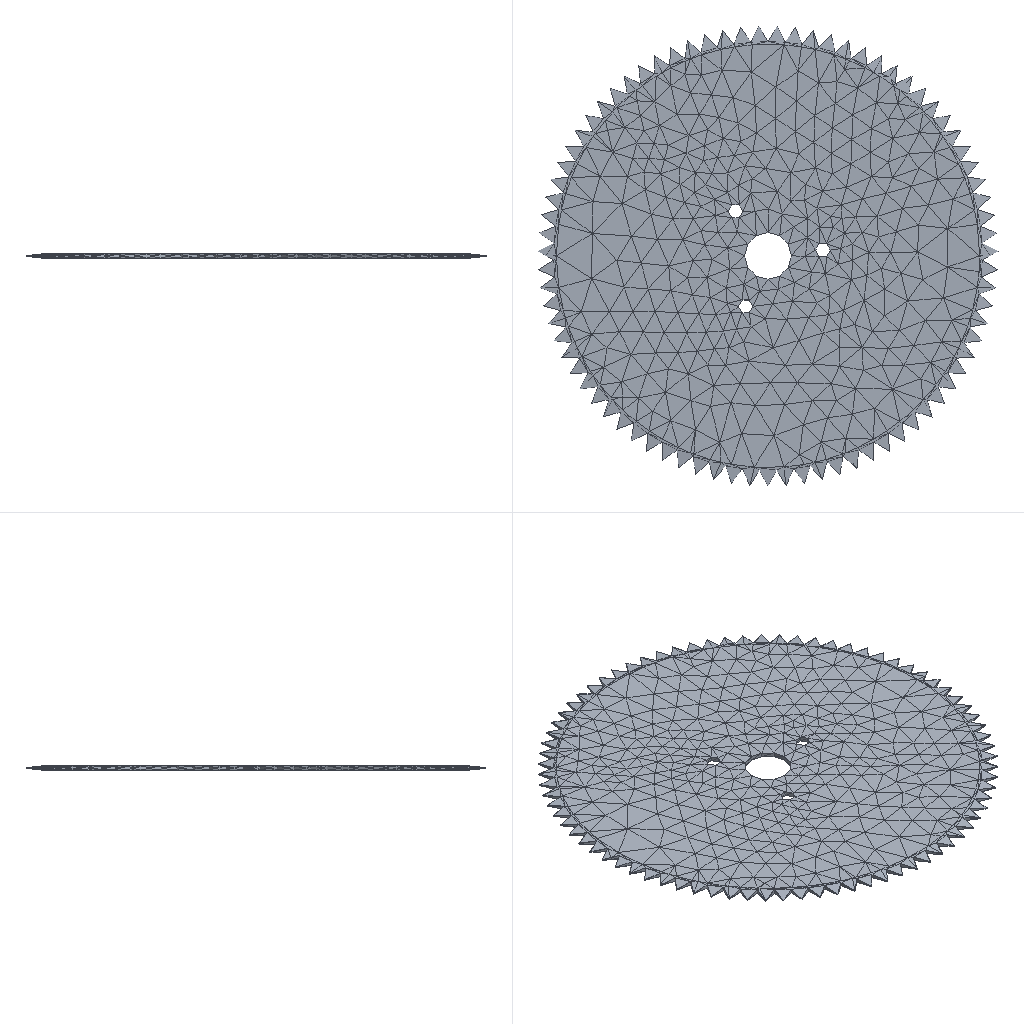Simulation study | ansys workbench
Set-up summary:
category,name,step,type,value,unit,region
solver,ansys_workbench
units,mm-N-s-tonne (MPa),,stated,"/units,MPA"
analysis,LS1,,modal,method=lanb; n_modes=6
load_step,LS1,LS1,modal
mesh,nodes,,,6469
mesh,elements,,,3002
element_type,SOLID187,,,3002
material,Structural Steel,,E,200000,tonne s^-2 mm^-1
material,Structural Steel,,nu,0.3
material,Structural Steel,,density,7.85e-09,tonne mm^-3
material,Structural Steel,,conductivity,60.5,tonne mm s^-3 C^-1
material,Structural Steel,,specific_heat,4.34e+08,mm^2 s^-2 C^-1
material,Structural Steel,,cte,1.2e-05,C^-1
material,Structural Steel,,permeability,10000
material,Structural Steel,,resistivity,0.00017,ohm mm
bc,Fixed Supports,model,fixed,[dofs=ALL],,_FIXEDSU
named_set,_FIXEDSU,,node,180
Ansys APDL input file, long lists of numbers shortened:
/batch
/config,noeldb,1     ! force off writing results to database
*get,_wallstrt,active,,time,wall
! ANSYS input file written by Workbench version 2022 R1
! File used for geometry attach:
/title,wbnew--__ (B5)
! ****** Begin Custom Load Command Snippet ******
/COM, ACT Extensions:
/COM,     LSDYNA, 2021.1
/COM,
! ****** End   Custom Load Command Snippet ******
*DIM,_wb_ProjectScratch_dir,string,248
_wb_ProjectScratch_dir(1) = ''
*DIM,_wb_SolverFiles_dir,string,248
_wb_SolverFiles_dir(1) = ''
*DIM,_wb_userfiles_dir,string,248
_wb_userfiles_dir(1) = ''
/com,--- Data in consistent NMM units. See Solving Units in the help system for more information.
/units,MPA
/nopr
/wb,file,start              !  signify a WB generated input file
/prep7
! Turn off shape checking because checks already performed inside WB mesher.
! See help system for more information.
SHPP,OFF,,NOWARN
/nolist
etcon,set             ! allow ANSYS to choose best KEYOP's for 180x elements, resets any applicable keyopt to MAPDL defaults
/com,*********** Nodes for the whole assembly ***********
nblock,3,,7115
(1i9,3e20.9e3)
        1    -1.150000000E+02     0.000000000E+00     2.500000000E+00
! (6468 more lines like these left out)
-1
/wb,elem,start            !  set before creation of elements
/com,*********** Elements for Body 1 "___-FreeParts|____(____)1" ***********
et,1,187
eblock,19,solid,,3002
(19i9)
        1        1        1        1        0        0        0        0       10        0        1      595      691      720     1005     4157     4945     4160     4166
! (6003 more lines like these left out)
-1
/wb,elem,end               !  done creating elements
/com,*********** Send User Defined Coordinate System(s) ***********
csys,0
toffst,273.15,  ! Temperature offset from absolute zero
/com,*********** Set Reference Temperature ***********
tref,22.
/wb,mat,start              !  starting to send materials
/com,*********** Send Materials ***********
Temperature = 'TEMP' ! Temperature
MP,DENS,1,7.85e-09,	! tonne mm^-3
MP,ALPX,1,1.2e-05,	! C^-1
MP,C,1,434000000,	! mm^2 s^-2 C^-1
MP,KXX,1,60.5,	! tonne mm s^-3 C^-1
MP,RSVX,1,0.00017,	! ohm mm
MP,EX,1,200000,	! tonne s^-2 mm^-1
MP,NUXY,1,0.3,
MP,MURX,1,10000,
/wb,mat,end                !  done sending materials
!************************* Model Summary ********************
!___-FreeParts|____(____)1,	结构钢,	matid,	1
!************************* End Model Summary ********************
! get the diagonal of the bounding box. Needed later for other things
*get,_xmin,node,,mnloc,x
*get,_ymin,node,,mnloc,y
*get,_zmin,node,,mnloc,z
*get,_xmax,node,,mxloc,x
*get,_ymax,node,,mxloc,y
*get,_zmax,node,,mxloc,z
_ASMDIAG=(_xmax-_xmin)*(_xmax-_xmin)+(_ymax-_ymin)*(_ymax-_ymin)+(_zmax-_zmin)*(_zmax-_zmin)
_ASMDIAG=SQRT(_ASMDIAG)
/wb,contact,start          !  starting to send contact
/wb,contact,end            !  done creating contacts
/golist
/wb,load,start             !  starting to send loads
/com,*********** Fixed Supports ***********
CMBLOCK,_FIXEDSU,NODE,      180
(8i10)
       207       208       209       210       211       212       213       214
! (22 more lines like these left out)
cmsel,s,_FIXEDSU
d,all,all
nsel,all
/gst,on,on
fini
*get,_numnode,node,0,count
*get,_numelem,elem,0,count
*get, _MAXELEMNUM, elem, 0, NUM, MAX
*get, _MAXNODENUM, node, 0, NUM, MAX
*get, _MAXELEMTYPE, etyp, 0, NUM, MAX
*get, _MAXREALCONST, real, 0, NUM, MAX
/go
/wb,load,end               !  done creating loads
/com,--- Number of total nodes = %_numnode%
/com,--- Number of contact elements = 0
/com,--- Number of spring elements = 0
/com,--- Number of bearing elements = 0
/com,--- Number of solid elements = 3002
/com,--- Number of condensed parts = 0
/com,--- Number of total elements = %_numelem%
*get,_wallbsol,active,,time,wall
/solu
antype,2                   ! modal analysis
_thickRatio=  0     ! Ratio of thick parts in the model
modopt,lanb,6
outres,erase
outres,all,none
outres,nsol,all
outres,etmp,all
mxpand                    ! default expand in case of complex solution
dmpopt,esav,no
dmpopt,emat,no
dmpopt,full,no
! *********** WB SOLVE COMMAND ***********
! check interactive state
*get,ANSINTER_,active,,int
*if,ANSINTER_,ne,0,then
/eof
*endif
solve
/com *************** Write FE CONNECTORS *********
CEWRITE,file,ce,,INTE
*get,_nmodalsolproc,active,0,numcpu
fini
/nopr
*get,_numnode,node,0,count
*get,_numelem,elem,0,count
*get, _MAXELEMNUM, elem, 0, NUM, MAX
*get, _MAXNODENUM, node, 0, NUM, MAX,,,INTERNAL
*get, _MAXELEMTYPE, etyp, 0, NUM, MAX
*get, _MAXREALCONST, real, 0, NUM, MAX
/gopr
*get,_wallasol,active,,time,wall
/post1
/nopr
*dim,_direction,CHAR,6,1
_direction(1) = 'X'
_direction(2) = 'Y'
_direction(3) = 'Z'
_direction(4) = 'ROTX'
_direction(5) = 'ROTY'
_direction(6) = 'ROTZ'
*get,_lastLS,active,0,set,LSTP
*get,_beginset,active,0,set,nset,first,_lastLS
*get,_endset,active,0,set,nset,last,_lastLS
_nummodes = 0
*if,_endset,gt,0,then
_nummodes = _endset - _beginset + 1
*endif
*do,i_mode,1,_nummodes
   *do,j_component,1,6
			*get,PFACT_%i_mode%_%j_component%,MODE,%i_mode%,PFACT,,DIREC,_direction(%j_component%)
   *enddo
*enddo
*dim,_tmdirection,CHAR,6,1
_tmdirection(1) = 'X'
_tmdirection(2) = 'Y'
_tmdirection(3) = 'Z'
_tmdirection(4) = 'X'
_tmdirection(5) = 'Y'
_tmdirection(6) = 'Z'
*do,j_component,1,6
    *if,j_component,gt,3,then
        *get,TOTALMASS_%j_component%,ELEM,0,IOR,_tmdirection(%j_component%)
    *else
        *get,TOTALMASS_%j_component%,ELEM,0,MTOT,_tmdirection(%j_component%)
    *endif
*enddo
/gopr
xmlo,ENCODING,ISO-8859-1
xmlo,parm
/xml,parm,xml
fini
/gopr
*get,_walldone,active,,time,wall
_preptime=(_wallbsol-_wallstrt)*3600
_solvtime=(_wallasol-_wallbsol)*3600
_posttime=(_walldone-_wallasol)*3600
_totaltim=(_walldone-_wallstrt)*3600
*get,_dlbratio,active,0,solu,dlbr
*get,_combtime,active,0,solu,comb
*get,_ssmode,active,0,solu,ssmm
*get,_ndofs,active,0,solu,ndof
/fclean				!clean distributed files
/com,--- Total number of nodes = %_numnode%
/com,--- Total number of elements = %_numelem%
/com,--- Element load balance ratio = %_dlbratio%
/com,--- Time to combine distributed files = %_combtime%
/com,--- Sparse memory mode = %_ssmode%
/com,--- Number of DOF = %_ndofs%
/wb,file,end               ! done with WB generated input
Results summary:
result,analyses[0].index,,,1
result,analyses[0].system,,,SYS
result,analyses[0].deck,,,deck.dat
result,analyses[0].solve_status,,,completed
result,analyses[0].analysis_type,,,modal
result,analyses[0].physics,,,mechanical
result,analyses[0].unit_system,,,"NMM: mm, ton, N, s, mV, mA, degC"
result,analyses[0].n_sets,,,6
result,analyses[0].modal_frequencies_hz[1],,,219.564
result,analyses[0].modal_frequencies_hz[2],,,220.903
result,analyses[0].modal_frequencies_hz[3],,,243.129
result,analyses[0].modal_frequencies_hz[4],,,297.649
result,analyses[0].modal_frequencies_hz[5],,,298.807
result,analyses[0].modal_frequencies_hz[6],,,537.101